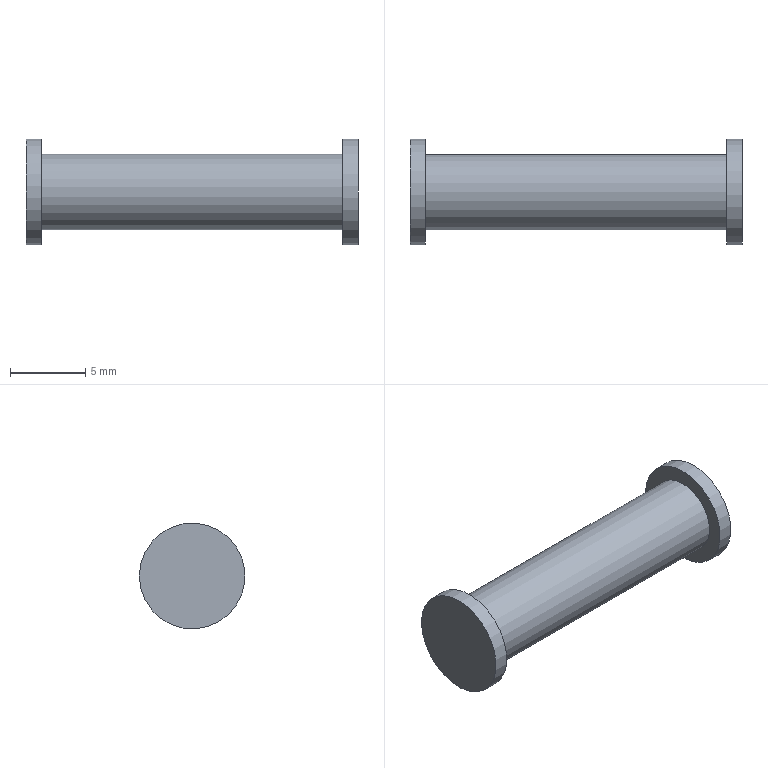Part | NX | features DATUM_CSYS 4, EXTRUDE 3, SKETCH 3 | 1 solid | 7 faces | box 22 x 7 x 7 mm | volume 469.668 mm3 | plane 4 | cylinder 3 | commonest cylinder face diameters 7 x2 5 x1
STEP:
#1=CARTESIAN_POINT('',(21.,0.,-2.5));
#2=VERTEX_POINT('',#1);
#3=CARTESIAN_POINT('',(21.,0.,0.));
#4=DIRECTION('',(1.,0.,0.));
#5=DIRECTION('',(0.,0.,-1.));
#6=AXIS2_PLACEMENT_3D('',#3,#4,#5);
#7=CIRCLE('',#6,2.5);
#8=EDGE_CURVE('',#2,#2,#7,.T.);
#9=ORIENTED_EDGE('',*,*,#8,.F.);
#10=EDGE_LOOP('',(#9));
#11=FACE_BOUND('',#10,.T.);
#12=CARTESIAN_POINT('',(1.,0.,2.5));
#13=VERTEX_POINT('',#12);
#14=CARTESIAN_POINT('',(1.,0.,0.));
#15=DIRECTION('',(-1.,0.,0.));
#16=DIRECTION('',(0.,0.,1.));
#17=AXIS2_PLACEMENT_3D('',#14,#15,#16);
#18=CIRCLE('',#17,2.5);
#19=EDGE_CURVE('',#13,#13,#18,.T.);
#20=ORIENTED_EDGE('',*,*,#19,.F.);
#21=EDGE_LOOP('',(#20));
#22=FACE_BOUND('',#21,.T.);
#23=CARTESIAN_POINT('',(22.,0.,0.));
#24=DIRECTION('',(-1.,0.,0.));
#25=DIRECTION('',(0.,0.,1.));
#26=AXIS2_PLACEMENT_3D('',#23,#24,#25);
#27=CYLINDRICAL_SURFACE('',#26,2.5);
#28=ADVANCED_FACE('',(#11,#22),#27,.T.);
#29=CARTESIAN_POINT('',(21.,3.5,0.));
#30=VERTEX_POINT('',#29);
#31=CARTESIAN_POINT('',(21.,0.,0.));
#32=DIRECTION('',(1.,0.,0.));
#33=DIRECTION('',(0.,1.,0.));
#34=AXIS2_PLACEMENT_3D('',#31,#32,#33);
#35=CIRCLE('',#34,3.5);
#36=EDGE_CURVE('',#30,#30,#35,.T.);
#37=ORIENTED_EDGE('',*,*,#36,.T.);
#38=EDGE_LOOP('',(#37));
#39=FACE_BOUND('',#38,.T.);
#40=CARTESIAN_POINT('',(22.,3.5,0.));
#41=VERTEX_POINT('',#40);
#42=CARTESIAN_POINT('',(22.,0.,0.));
#43=DIRECTION('',(1.,0.,0.));
#44=DIRECTION('',(0.,1.,0.));
#45=AXIS2_PLACEMENT_3D('',#42,#43,#44);
#46=CIRCLE('',#45,3.5);
#47=EDGE_CURVE('',#41,#41,#46,.T.);
#48=ORIENTED_EDGE('',*,*,#47,.F.);
#49=EDGE_LOOP('',(#48));
#50=FACE_BOUND('',#49,.T.);
#51=CARTESIAN_POINT('',(21.,0.,0.));
#52=DIRECTION('',(1.,0.,0.));
#53=DIRECTION('',(0.,0.,-1.));
#54=AXIS2_PLACEMENT_3D('',#51,#52,#53);
#55=CYLINDRICAL_SURFACE('',#54,3.5);
#56=ADVANCED_FACE('',(#39,#50),#55,.T.);
#57=ORIENTED_EDGE('',*,*,#8,.T.);
#58=EDGE_LOOP('',(#57));
#59=FACE_BOUND('',#58,.T.);
#60=ORIENTED_EDGE('',*,*,#36,.F.);
#61=EDGE_LOOP('',(#60));
#62=FACE_BOUND('',#61,.T.);
#63=CARTESIAN_POINT('',(21.,0.,0.));
#64=DIRECTION('',(1.,0.,0.));
#65=DIRECTION('',(0.,0.,-1.));
#66=AXIS2_PLACEMENT_3D('',#63,#64,#65);
#67=PLANE('',#66);
#68=ADVANCED_FACE('',(#59,#62),#67,.F.);
#69=ORIENTED_EDGE('',*,*,#47,.T.);
#70=EDGE_LOOP('',(#69));
#71=FACE_BOUND('',#70,.T.);
#72=CARTESIAN_POINT('',(22.,0.,0.));
#73=DIRECTION('',(1.,0.,0.));
#74=DIRECTION('',(0.,0.,-1.));
#75=AXIS2_PLACEMENT_3D('',#72,#73,#74);
#76=PLANE('',#75);
#77=ADVANCED_FACE('',(#71),#76,.T.);
#78=CARTESIAN_POINT('',(1.,3.5,0.));
#79=VERTEX_POINT('',#78);
#80=CARTESIAN_POINT('',(1.,0.,0.));
#81=DIRECTION('',(-1.,0.,0.));
#82=DIRECTION('',(0.,1.,0.));
#83=AXIS2_PLACEMENT_3D('',#80,#81,#82);
#84=CIRCLE('',#83,3.5);
#85=EDGE_CURVE('',#79,#79,#84,.T.);
#86=ORIENTED_EDGE('',*,*,#85,.T.);
#87=EDGE_LOOP('',(#86));
#88=FACE_BOUND('',#87,.T.);
#89=CARTESIAN_POINT('',(0.,3.5,0.));
#90=VERTEX_POINT('',#89);
#91=CARTESIAN_POINT('',(0.,0.,0.));
#92=DIRECTION('',(-1.,0.,0.));
#93=DIRECTION('',(0.,1.,0.));
#94=AXIS2_PLACEMENT_3D('',#91,#92,#93);
#95=CIRCLE('',#94,3.5);
#96=EDGE_CURVE('',#90,#90,#95,.T.);
#97=ORIENTED_EDGE('',*,*,#96,.F.);
#98=EDGE_LOOP('',(#97));
#99=FACE_BOUND('',#98,.T.);
#100=CARTESIAN_POINT('',(1.,0.,0.));
#101=DIRECTION('',(-1.,0.,0.));
#102=DIRECTION('',(0.,0.,1.));
#103=AXIS2_PLACEMENT_3D('',#100,#101,#102);
#104=CYLINDRICAL_SURFACE('',#103,3.5);
#105=ADVANCED_FACE('',(#88,#99),#104,.T.);
#106=ORIENTED_EDGE('',*,*,#19,.T.);
#107=EDGE_LOOP('',(#106));
#108=FACE_BOUND('',#107,.T.);
#109=ORIENTED_EDGE('',*,*,#85,.F.);
#110=EDGE_LOOP('',(#109));
#111=FACE_BOUND('',#110,.T.);
#112=CARTESIAN_POINT('',(1.,0.,0.));
#113=DIRECTION('',(-1.,0.,0.));
#114=DIRECTION('',(0.,0.,1.));
#115=AXIS2_PLACEMENT_3D('',#112,#113,#114);
#116=PLANE('',#115);
#117=ADVANCED_FACE('',(#108,#111),#116,.F.);
#118=ORIENTED_EDGE('',*,*,#96,.T.);
#119=EDGE_LOOP('',(#118));
#120=FACE_BOUND('',#119,.T.);
#121=CARTESIAN_POINT('',(0.,0.,0.));
#122=DIRECTION('',(1.,0.,0.));
#123=DIRECTION('',(0.,0.,-1.));
#124=AXIS2_PLACEMENT_3D('',#121,#122,#123);
#125=PLANE('',#124);
#126=ADVANCED_FACE('',(#120),#125,.F.);
#127=CLOSED_SHELL('',(#28,#56,#68,#77,#105,#117,#126));
#128=MANIFOLD_SOLID_BREP('',#127);
#129=(LENGTH_UNIT()NAMED_UNIT(*)SI_UNIT(.MILLI.,.METRE.));
#130=UNCERTAINTY_MEASURE_WITH_UNIT(LENGTH_MEASURE(0.00001),#129,'','');
#131=(NAMED_UNIT(*)PLANE_ANGLE_UNIT()SI_UNIT($,.RADIAN.));
#132=(NAMED_UNIT(*)SI_UNIT($,.STERADIAN.)SOLID_ANGLE_UNIT());
#133=(GEOMETRIC_REPRESENTATION_CONTEXT(3)GLOBAL_UNCERTAINTY_ASSIGNED_CONTEXT((#130))GLOBAL_UNIT_ASSIGNED_CONTEXT((#129,#131,#132))REPRESENTATION_CONTEXT('',''));
#134=ADVANCED_BREP_SHAPE_REPRESENTATION('',(#128),#133);